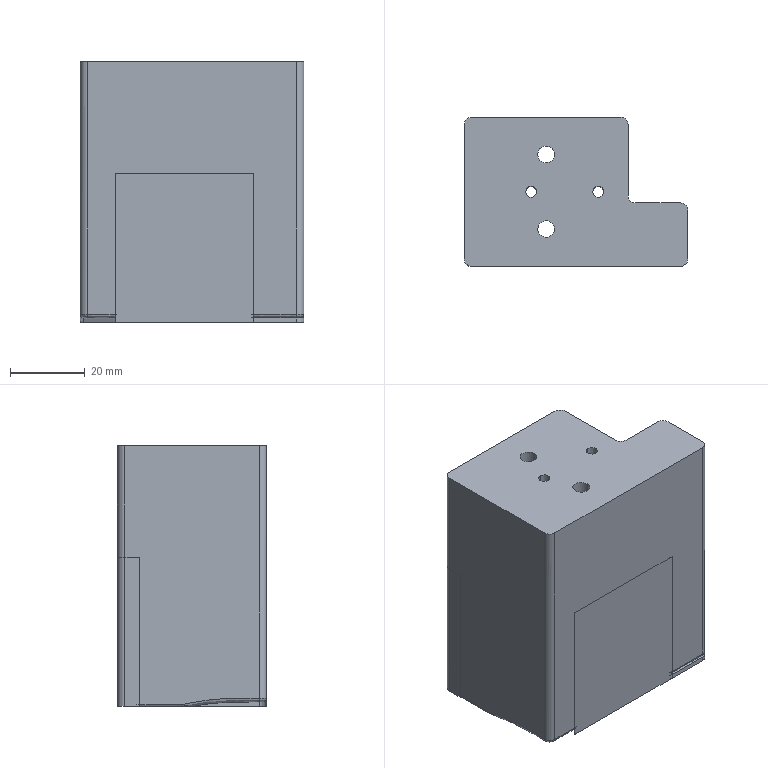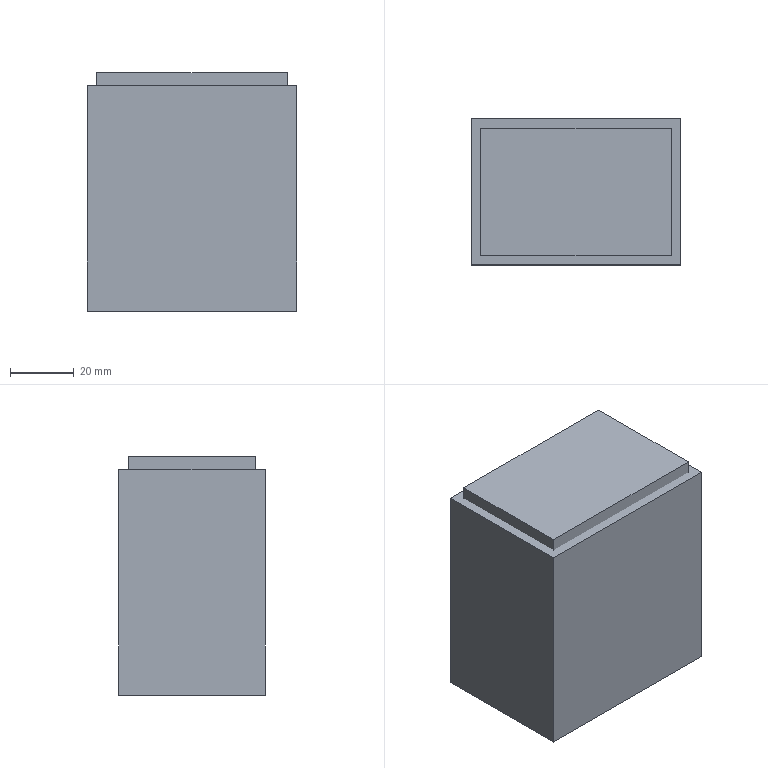CAM job | NX | 3+2 milling, drilling | part box 60.004 x 40.015 x 70 mm | stock box 66.004 x 46.015 x 75 mm
Tools:
number,name,description,diameter,corner_radius,flute_length,length,flutes
1,D63,Milling Tool-5 Parameters,63.0,0.0,50.0,75.0,2
9,D10,Milling Tool-5 Parameters,10.0,0.0,50.0,75.0,2
10,D10JING,Milling Tool-5 Parameters,10.0,0.0,50.0,75.0,2
8,D6R0.5,Milling Tool-5 Parameters,6.0,0.5,50.0,75.0,2
2,D4A45,Milling Tool-5 Parameters,4.0,0.0,2.0,2.0,2
15,4.5ZT,Drilling Tool,4.5,0.0,35.0,50.0,2
13,3.0ZT,Drilling Tool,3.0,0.0,35.0,50.0,2
7,D8,Milling Tool-5 Parameters,8.0,0.0,50.0,75.0,2
Operations:
program,operation,operation_type,tool,method,geometry_group,spindle_rpm,surface_speed,feed_per_tooth,feed_cut,feed_plunge,cut_length_mm,path_length_mm,cut_time_min,machine_time_min
1,FLOOR_WALL,VolumeBased25DMillingOperation,D63,METHOD,A,6500.0,1286.0,0.0962,1250.0,100.0,469.8,523.801,0.3758,0.3812
1,CAVITY_MILL,CavityMilling,D10,METHOD,A,9500.0,298.0,0.1579,3000.0,1000.0,22247.772,22527.592,7.613,7.641
1,ZLEVEL_PROFILE_COPY_COPY,ZLevelMilling,D10JING,METHOD,A,9500.0,119.0,0.0632,1200.0,1000.0,599.513,836.872,0.5009,0.5247
1,ZLEVEL_PROFILE_COPY_COPY_COPY,ZLevelMilling,D10JING,METHOD,A,9500.0,119.0,0.0632,1200.0,1000.0,267.754,366.754,0.2238,0.2337
1,FLOOR_WALL_1,VolumeBased25DMillingOperation,D10JING,METHOD,A,9500.0,119.0,0.0526,1000.0,100.0,339.635,628.637,0.3396,0.3685
1,ZLEVEL_PROFILE_COPY,ZLevelMilling,D6R0.5,METHOD,A,9500.0,179.0,0.1579,3000.0,1000.0,6301.25,6470.013,2.104,2.121
1,ZLEVEL_PROFILE_COPY_COPY_1,ZLevelMilling,D6R0.5,METHOD,A,9500.0,179.0,0.1579,3000.0,1000.0,2382.622,2483.722,0.7962,0.8063
1,ZLEVEL_PROFILE_COPY_COPY_1_COPY,ZLevelMilling,D6R0.5,METHOD,A,9500.0,179.0,0.1579,3000.0,1000.0,4173.941,4911.49,1.403,1.477
2,FLOOR_WALL_COPY,VolumeBased25DMillingOperation,D63,METHOD,B,6500.0,1286.0,0.0962,1250.0,100.0,2674.803,3690.18,2.14,2.241
2,ZLEVEL_PROFILE_COPY_COPY_2,ZLevelMilling,D6R0.5,METHOD,B,9500.0,179.0,0.1579,3000.0,1000.0,6269.895,6489.626,2.094,2.116
3,DRILLING_COPY,Operation,D4A45,METHOD,C,5000.0,62.0,0.025,250.0,0.0,16.0,156.936,0.064,0.0781
3,DRILLING_COPY_COPY_COPY_COPY_COPY,Operation,3.0ZT,METHOD,C,1910.0,21.0,0.0471,180.0,0.0,70.803,222.853,0.3933,0.4086
3,DRILLING_COPY_COPY_COPY_COPY_COPY_COPY,Operation,4.5ZT,METHOD,C,1910.0,21.0,0.0471,180.0,0.0,70.704,224.631,0.3928,0.4082
3,ZLEVEL_PROFILE_1_COPY_1_COPY_COPY,ZLevelMilling,D4A45,METHOD,C,9500.0,179.0,0.0526,1000.0,100.0,243.189,622.76,0.2432,0.2811
4,FLOOR_WALL_2,VolumeBased25DMillingOperation,D10,METHOD,D,9500.0,298.0,0.1316,2500.0,1000.0,17873.512,18603.073,7.238,7.311
4,FLOOR_WALL_1_COPY_COPY,VolumeBased25DMillingOperation,D10JING,METHOD,D,9500.0,119.0,0.0526,1000.0,100.0,235.301,841.968,0.2353,0.296
4,FLOOR_WALL_1_COPY,VolumeBased25DMillingOperation,D10JING,METHOD,D,9500.0,119.0,0.0526,1000.0,100.0,478.56,1513.137,0.4786,0.582
4,DRILLING_COPY_COPY_COPY_COPY_COPY_COPY_COPY,Operation,D8,METHOD,D,1500.0,37.0,0.06,180.0,0.0,36.0,235.224,0.2,0.2199
4,FIXED_CONTOUR,SurfaceContour,D6R0.5,METHOD,D,9500.0,179.0,0.1316,2500.0,1000.0,15173.776,15353.745,6.084,6.102